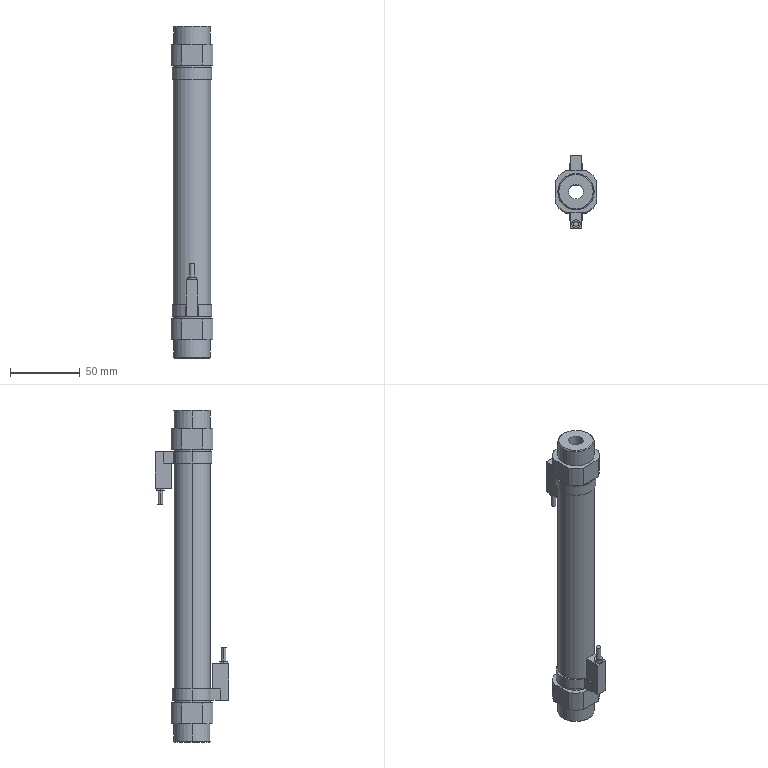Part | STEP file | body_A_CDM2WB25_150_C76_0_ | 1 solid | 97 faces | box 30 x 52.6 x 238 mm | volume 124557 mm3 | plane 49 | cylinder 40 | cone 8 | commonest cylinder face diameters 28.6 x8 33.5 x8 26.6 x6 3.4 x4 6 x4 8.57 x4